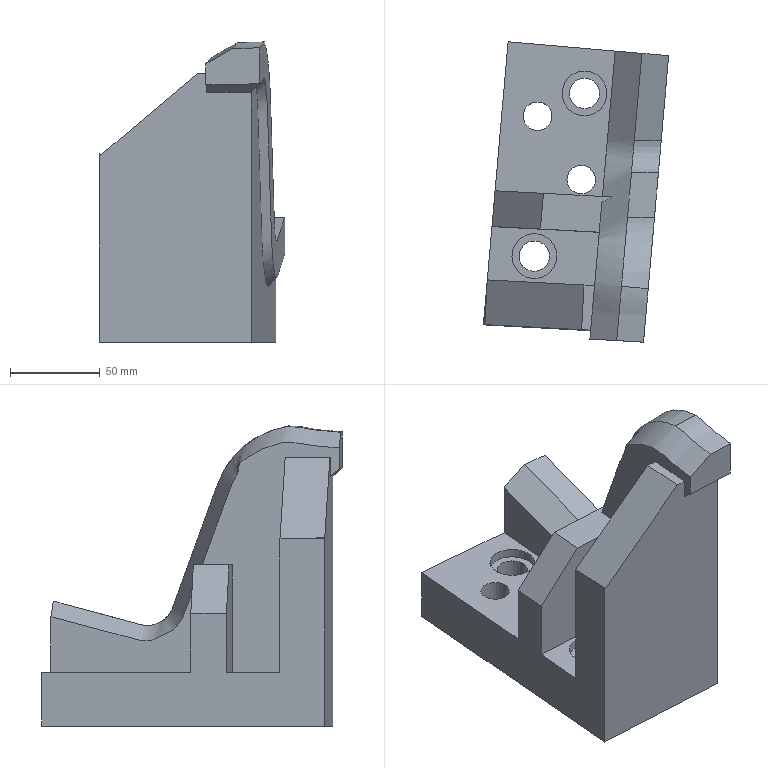Part | NX | features solid 2 | 1 solid | 36 faces | box 103.489 x 168.016 x 167.665 mm | volume 908681 mm3 | plane 15 | spline 15 | cylinder 6 | commonest cylinder face diameters 16 x2 17 x2 25 x2